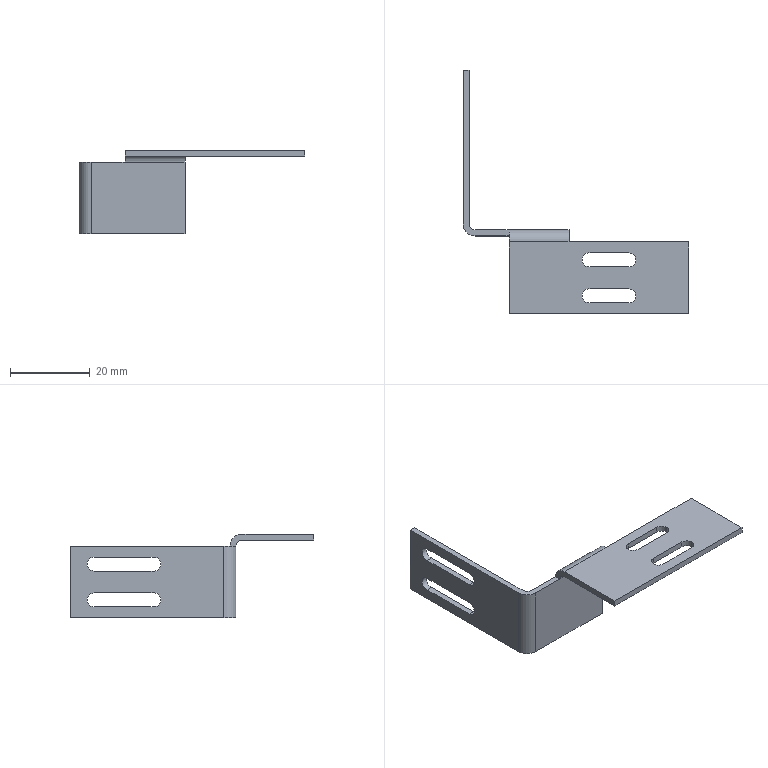Part | SolidWorks | features ICE 4, Fillet 2, ExtruThin 1 | 1 solid | 36 faces | box 56.5 x 61 x 21 mm | volume 2744 mm3 | plane 22 | cylinder 14 | commonest cylinder face diameters 3.5 x10 3 x2 6 x2
STEP:
#1=CARTESIAN_POINT('',(40.,-14.75,19.5));
#2=VERTEX_POINT('',#1);
#3=CARTESIAN_POINT('',(41.75,-16.5,19.5));
#4=VERTEX_POINT('',#3);
#5=CARTESIAN_POINT('',(40.,-16.5,19.5));
#6=DIRECTION('',(0.,0.,-1.));
#7=DIRECTION('',(0.,1.,0.));
#8=AXIS2_PLACEMENT_3D('',#5,#6,#7);
#9=CIRCLE('',#8,1.75);
#10=EDGE_CURVE('',#2,#4,#9,.T.);
#11=ORIENTED_EDGE('',*,*,#10,.T.);
#12=CARTESIAN_POINT('',(41.75,-16.5,21.));
#13=VERTEX_POINT('',#12);
#14=CARTESIAN_POINT('',(41.75,-16.5,11.));
#15=DIRECTION('',(0.,0.,1.));
#16=VECTOR('',#15,1000.);
#17=LINE('',#14,#16);
#18=EDGE_CURVE('',#4,#13,#17,.T.);
#19=ORIENTED_EDGE('',*,*,#18,.T.);
#20=CARTESIAN_POINT('',(40.,-14.75,21.));
#21=VERTEX_POINT('',#20);
#22=CARTESIAN_POINT('',(40.,-16.5,21.));
#23=DIRECTION('',(0.,0.,1.));
#24=DIRECTION('',(-1.,0.,0.));
#25=AXIS2_PLACEMENT_3D('',#22,#23,#24);
#26=CIRCLE('',#25,1.75);
#27=EDGE_CURVE('',#13,#21,#26,.T.);
#28=ORIENTED_EDGE('',*,*,#27,.T.);
#29=CARTESIAN_POINT('',(40.,-14.75,11.));
#30=DIRECTION('',(0.,0.,1.));
#31=VECTOR('',#30,1000.);
#32=LINE('',#29,#31);
#33=EDGE_CURVE('',#2,#21,#32,.T.);
#34=ORIENTED_EDGE('',*,*,#33,.F.);
#35=EDGE_LOOP('',(#11,#19,#28,#34));
#36=FACE_OUTER_BOUND('',#35,.T.);
#37=CARTESIAN_POINT('',(40.,-16.5,11.));
#38=DIRECTION('',(0.,0.,1.));
#39=DIRECTION('',(1.,0.,0.));
#40=AXIS2_PLACEMENT_3D('',#37,#38,#39);
#41=CYLINDRICAL_SURFACE('',#40,1.75);
#42=ADVANCED_FACE('',(#36),#41,.F.);
#43=CARTESIAN_POINT('',(40.,-5.75,19.5));
#44=VERTEX_POINT('',#43);
#45=CARTESIAN_POINT('',(41.75,-7.5,19.5));
#46=VERTEX_POINT('',#45);
#47=CARTESIAN_POINT('',(40.,-7.5,19.5));
#48=DIRECTION('',(0.,0.,-1.));
#49=DIRECTION('',(0.,1.,0.));
#50=AXIS2_PLACEMENT_3D('',#47,#48,#49);
#51=CIRCLE('',#50,1.75);
#52=EDGE_CURVE('',#44,#46,#51,.T.);
#53=ORIENTED_EDGE('',*,*,#52,.T.);
#54=CARTESIAN_POINT('',(41.75,-7.5,21.));
#55=VERTEX_POINT('',#54);
#56=CARTESIAN_POINT('',(41.75,-7.5,11.));
#57=DIRECTION('',(0.,0.,1.));
#58=VECTOR('',#57,1000.);
#59=LINE('',#56,#58);
#60=EDGE_CURVE('',#46,#55,#59,.T.);
#61=ORIENTED_EDGE('',*,*,#60,.T.);
#62=CARTESIAN_POINT('',(40.,-5.75,21.));
#63=VERTEX_POINT('',#62);
#64=CARTESIAN_POINT('',(40.,-7.5,21.));
#65=DIRECTION('',(0.,0.,1.));
#66=DIRECTION('',(1.,0.,0.));
#67=AXIS2_PLACEMENT_3D('',#64,#65,#66);
#68=CIRCLE('',#67,1.75);
#69=EDGE_CURVE('',#55,#63,#68,.T.);
#70=ORIENTED_EDGE('',*,*,#69,.T.);
#71=CARTESIAN_POINT('',(40.,-5.75,11.));
#72=DIRECTION('',(0.,0.,1.));
#73=VECTOR('',#72,1000.);
#74=LINE('',#71,#73);
#75=EDGE_CURVE('',#44,#63,#74,.T.);
#76=ORIENTED_EDGE('',*,*,#75,.F.);
#77=EDGE_LOOP('',(#53,#61,#70,#76));
#78=FACE_OUTER_BOUND('',#77,.T.);
#79=CARTESIAN_POINT('',(40.,-7.5,11.));
#80=DIRECTION('',(0.,0.,1.));
#81=DIRECTION('',(1.,0.,0.));
#82=AXIS2_PLACEMENT_3D('',#79,#80,#81);
#83=CYLINDRICAL_SURFACE('',#82,1.75);
#84=ADVANCED_FACE('',(#78),#83,.F.);
#85=CARTESIAN_POINT('',(10.,-3.,21.));
#86=VERTEX_POINT('',#85);
#87=CARTESIAN_POINT('',(25.,-3.,21.));
#88=VERTEX_POINT('',#87);
#89=CARTESIAN_POINT('',(10.,-3.,21.));
#90=DIRECTION('',(1.,0.,0.));
#91=VECTOR('',#90,1000.);
#92=LINE('',#89,#91);
#93=EDGE_CURVE('',#86,#88,#92,.T.);
#94=ORIENTED_EDGE('',*,*,#93,.T.);
#95=CARTESIAN_POINT('',(25.,0.,18.));
#96=VERTEX_POINT('',#95);
#97=CARTESIAN_POINT('',(25.,-3.,18.));
#98=DIRECTION('',(-1.,0.,0.));
#99=DIRECTION('',(0.,0.,-1.));
#100=AXIS2_PLACEMENT_3D('',#97,#98,#99);
#101=CIRCLE('',#100,3.);
#102=EDGE_CURVE('',#88,#96,#101,.T.);
#103=ORIENTED_EDGE('',*,*,#102,.T.);
#104=CARTESIAN_POINT('',(10.,0.,18.));
#105=VERTEX_POINT('',#104);
#106=CARTESIAN_POINT('',(10.,0.,18.));
#107=DIRECTION('',(1.,0.,0.));
#108=VECTOR('',#107,1000.);
#109=LINE('',#106,#108);
#110=EDGE_CURVE('',#105,#96,#109,.T.);
#111=ORIENTED_EDGE('',*,*,#110,.F.);
#112=CARTESIAN_POINT('',(10.,-3.,18.));
#113=DIRECTION('',(1.,0.,0.));
#114=DIRECTION('',(0.,0.,-1.));
#115=AXIS2_PLACEMENT_3D('',#112,#113,#114);
#116=CIRCLE('',#115,3.);
#117=EDGE_CURVE('',#105,#86,#116,.T.);
#118=ORIENTED_EDGE('',*,*,#117,.T.);
#119=EDGE_LOOP('',(#94,#103,#111,#118));
#120=FACE_OUTER_BOUND('',#119,.T.);
#121=CARTESIAN_POINT('',(10.,-3.,18.));
#122=DIRECTION('',(1.,0.,0.));
#123=DIRECTION('',(0.,0.,-1.));
#124=AXIS2_PLACEMENT_3D('',#121,#122,#123);
#125=CYLINDRICAL_SURFACE('',#124,3.);
#126=ADVANCED_FACE('',(#120),#125,.T.);
#127=CARTESIAN_POINT('',(10.,-1.5,18.));
#128=VERTEX_POINT('',#127);
#129=CARTESIAN_POINT('',(25.,-1.5,18.));
#130=VERTEX_POINT('',#129);
#131=CARTESIAN_POINT('',(10.,-1.5,18.));
#132=DIRECTION('',(1.,0.,0.));
#133=VECTOR('',#132,1000.);
#134=LINE('',#131,#133);
#135=EDGE_CURVE('',#128,#130,#134,.T.);
#136=ORIENTED_EDGE('',*,*,#135,.T.);
#137=CARTESIAN_POINT('',(25.,-3.,19.5));
#138=VERTEX_POINT('',#137);
#139=CARTESIAN_POINT('',(25.,-3.,18.));
#140=DIRECTION('',(1.,0.,0.));
#141=DIRECTION('',(0.,0.,-1.));
#142=AXIS2_PLACEMENT_3D('',#139,#140,#141);
#143=CIRCLE('',#142,1.5);
#144=EDGE_CURVE('',#130,#138,#143,.T.);
#145=ORIENTED_EDGE('',*,*,#144,.T.);
#146=CARTESIAN_POINT('',(10.,-3.,19.5));
#147=VERTEX_POINT('',#146);
#148=CARTESIAN_POINT('',(10.,-3.,19.5));
#149=DIRECTION('',(1.,0.,0.));
#150=VECTOR('',#149,1000.);
#151=LINE('',#148,#150);
#152=EDGE_CURVE('',#147,#138,#151,.T.);
#153=ORIENTED_EDGE('',*,*,#152,.F.);
#154=CARTESIAN_POINT('',(10.,-3.,18.));
#155=DIRECTION('',(-1.,0.,0.));
#156=DIRECTION('',(0.,0.,-1.));
#157=AXIS2_PLACEMENT_3D('',#154,#155,#156);
#158=CIRCLE('',#157,1.5);
#159=EDGE_CURVE('',#147,#128,#158,.T.);
#160=ORIENTED_EDGE('',*,*,#159,.T.);
#161=EDGE_LOOP('',(#136,#145,#153,#160));
#162=FACE_OUTER_BOUND('',#161,.T.);
#163=CARTESIAN_POINT('',(10.,-3.,18.));
#164=DIRECTION('',(1.,0.,0.));
#165=DIRECTION('',(0.,0.,-1.));
#166=AXIS2_PLACEMENT_3D('',#163,#164,#165);
#167=CYLINDRICAL_SURFACE('',#166,1.5);
#168=ADVANCED_FACE('',(#162),#167,.F.);
#169=CARTESIAN_POINT('',(1.5,-1.5,18.));
#170=VERTEX_POINT('',#169);
#171=CARTESIAN_POINT('',(0.,-1.5,18.));
#172=DIRECTION('',(1.,0.,0.));
#173=VECTOR('',#172,1000.);
#174=LINE('',#171,#173);
#175=EDGE_CURVE('',#170,#128,#174,.T.);
#176=ORIENTED_EDGE('',*,*,#175,.F.);
#177=CARTESIAN_POINT('',(1.5,-1.5,0.));
#178=VERTEX_POINT('',#177);
#179=CARTESIAN_POINT('',(1.5,-1.5,18.));
#180=DIRECTION('',(0.,0.,-1.));
#181=VECTOR('',#180,1000.);
#182=LINE('',#179,#181);
#183=EDGE_CURVE('',#170,#178,#182,.T.);
#184=ORIENTED_EDGE('',*,*,#183,.T.);
#185=CARTESIAN_POINT('',(25.,-1.5,0.));
#186=VERTEX_POINT('',#185);
#187=CARTESIAN_POINT('',(0.,-1.5,0.));
#188=DIRECTION('',(1.,0.,0.));
#189=VECTOR('',#188,1000.);
#190=LINE('',#187,#189);
#191=EDGE_CURVE('',#178,#186,#190,.T.);
#192=ORIENTED_EDGE('',*,*,#191,.T.);
#193=CARTESIAN_POINT('',(25.,-1.5,18.));
#194=DIRECTION('',(0.,0.,-1.));
#195=VECTOR('',#194,1000.);
#196=LINE('',#193,#195);
#197=EDGE_CURVE('',#130,#186,#196,.T.);
#198=ORIENTED_EDGE('',*,*,#197,.F.);
#199=ORIENTED_EDGE('',*,*,#135,.F.);
#200=EDGE_LOOP('',(#176,#184,#192,#198,#199));
#201=FACE_OUTER_BOUND('',#200,.T.);
#202=CARTESIAN_POINT('',(0.,-1.5,18.));
#203=DIRECTION('',(0.,1.,0.));
#204=DIRECTION('',(0.,0.,1.));
#205=AXIS2_PLACEMENT_3D('',#202,#203,#204);
#206=PLANE('',#205);
#207=ADVANCED_FACE('',(#201),#206,.F.);
#208=CARTESIAN_POINT('',(25.,0.,0.));
#209=VERTEX_POINT('',#208);
#210=CARTESIAN_POINT('',(25.,0.,0.));
#211=DIRECTION('',(0.,-1.,0.));
#212=VECTOR('',#211,1000.);
#213=LINE('',#210,#212);
#214=EDGE_CURVE('',#209,#186,#213,.T.);
#215=ORIENTED_EDGE('',*,*,#214,.F.);
#216=CARTESIAN_POINT('',(25.,0.,18.));
#217=DIRECTION('',(0.,0.,-1.));
#218=VECTOR('',#217,1000.);
#219=LINE('',#216,#218);
#220=EDGE_CURVE('',#96,#209,#219,.T.);
#221=ORIENTED_EDGE('',*,*,#220,.F.);
#222=ORIENTED_EDGE('',*,*,#102,.F.);
#223=CARTESIAN_POINT('',(25.,-3.,21.));
#224=DIRECTION('',(0.,0.,1.));
#225=VECTOR('',#224,1000.);
#226=LINE('',#223,#225);
#227=EDGE_CURVE('',#138,#88,#226,.T.);
#228=ORIENTED_EDGE('',*,*,#227,.F.);
#229=ORIENTED_EDGE('',*,*,#144,.F.);
#230=ORIENTED_EDGE('',*,*,#197,.T.);
#231=EDGE_LOOP('',(#215,#221,#222,#228,#229,#230));
#232=FACE_OUTER_BOUND('',#231,.T.);
#233=CARTESIAN_POINT('',(25.,0.,18.));
#234=DIRECTION('',(1.,0.,0.));
#235=DIRECTION('',(0.,0.,-1.));
#236=AXIS2_PLACEMENT_3D('',#233,#234,#235);
#237=PLANE('',#236);
#238=ADVANCED_FACE('',(#232),#237,.T.);
#239=CARTESIAN_POINT('',(1.5,0.,0.));
#240=VERTEX_POINT('',#239);
#241=CARTESIAN_POINT('',(0.,0.,0.));
#242=DIRECTION('',(1.,0.,0.));
#243=VECTOR('',#242,1000.);
#244=LINE('',#241,#243);
#245=EDGE_CURVE('',#240,#209,#244,.T.);
#246=ORIENTED_EDGE('',*,*,#245,.F.);
#247=CARTESIAN_POINT('',(1.5,0.,18.));
#248=VERTEX_POINT('',#247);
#249=CARTESIAN_POINT('',(1.5,0.,18.));
#250=DIRECTION('',(0.,0.,1.));
#251=VECTOR('',#250,1000.);
#252=LINE('',#249,#251);
#253=EDGE_CURVE('',#240,#248,#252,.T.);
#254=ORIENTED_EDGE('',*,*,#253,.T.);
#255=CARTESIAN_POINT('',(0.,0.,18.));
#256=DIRECTION('',(1.,0.,0.));
#257=VECTOR('',#256,1000.);
#258=LINE('',#255,#257);
#259=EDGE_CURVE('',#248,#105,#258,.T.);
#260=ORIENTED_EDGE('',*,*,#259,.T.);
#261=ORIENTED_EDGE('',*,*,#110,.T.);
#262=ORIENTED_EDGE('',*,*,#220,.T.);
#263=EDGE_LOOP('',(#246,#254,#260,#261,#262));
#264=FACE_OUTER_BOUND('',#263,.T.);
#265=CARTESIAN_POINT('',(0.,0.,18.));
#266=DIRECTION('',(0.,1.,0.));
#267=DIRECTION('',(0.,0.,1.));
#268=AXIS2_PLACEMENT_3D('',#265,#266,#267);
#269=PLANE('',#268);
#270=ADVANCED_FACE('',(#264),#269,.T.);
#271=CARTESIAN_POINT('',(0.,34.,11.75));
#272=VERTEX_POINT('',#271);
#273=CARTESIAN_POINT('',(0.,34.,15.25));
#274=VERTEX_POINT('',#273);
#275=CARTESIAN_POINT('',(0.,34.,13.5));
#276=DIRECTION('',(1.,0.,0.));
#277=DIRECTION('',(0.,0.,-1.));
#278=AXIS2_PLACEMENT_3D('',#275,#276,#277);
#279=CIRCLE('',#278,1.75);
#280=EDGE_CURVE('',#272,#274,#279,.T.);
#281=ORIENTED_EDGE('',*,*,#280,.F.);
#282=CARTESIAN_POINT('',(0.,19.,11.75));
#283=VERTEX_POINT('',#282);
#284=CARTESIAN_POINT('',(0.,0.,11.75));
#285=DIRECTION('',(0.,1.,0.));
#286=VECTOR('',#285,1000.);
#287=LINE('',#284,#286);
#288=EDGE_CURVE('',#283,#272,#287,.T.);
#289=ORIENTED_EDGE('',*,*,#288,.F.);
#290=CARTESIAN_POINT('',(0.,19.,15.25));
#291=VERTEX_POINT('',#290);
#292=CARTESIAN_POINT('',(0.,19.,13.5));
#293=DIRECTION('',(1.,0.,0.));
#294=DIRECTION('',(0.,0.,-1.));
#295=AXIS2_PLACEMENT_3D('',#292,#293,#294);
#296=CIRCLE('',#295,1.75);
#297=EDGE_CURVE('',#291,#283,#296,.T.);
#298=ORIENTED_EDGE('',*,*,#297,.F.);
#299=CARTESIAN_POINT('',(0.,0.,15.25));
#300=DIRECTION('',(0.,-1.,0.));
#301=VECTOR('',#300,1000.);
#302=LINE('',#299,#301);
#303=EDGE_CURVE('',#274,#291,#302,.T.);
#304=ORIENTED_EDGE('',*,*,#303,.F.);
#305=EDGE_LOOP('',(#281,#289,#298,#304));
#306=FACE_BOUND('',#305,.T.);
#307=CARTESIAN_POINT('',(0.,34.,2.75));
#308=VERTEX_POINT('',#307);
#309=CARTESIAN_POINT('',(0.,34.,6.25));
#310=VERTEX_POINT('',#309);
#311=CARTESIAN_POINT('',(0.,34.,4.5));
#312=DIRECTION('',(1.,0.,0.));
#313=DIRECTION('',(0.,0.,-1.));
#314=AXIS2_PLACEMENT_3D('',#311,#312,#313);
#315=CIRCLE('',#314,1.75);
#316=EDGE_CURVE('',#308,#310,#315,.T.);
#317=ORIENTED_EDGE('',*,*,#316,.F.);
#318=CARTESIAN_POINT('',(0.,19.,2.75));
#319=VERTEX_POINT('',#318);
#320=CARTESIAN_POINT('',(0.,0.,2.75));
#321=DIRECTION('',(0.,1.,0.));
#322=VECTOR('',#321,1000.);
#323=LINE('',#320,#322);
#324=EDGE_CURVE('',#319,#308,#323,.T.);
#325=ORIENTED_EDGE('',*,*,#324,.F.);
#326=CARTESIAN_POINT('',(0.,19.,6.25));
#327=VERTEX_POINT('',#326);
#328=CARTESIAN_POINT('',(0.,19.,4.5));
#329=DIRECTION('',(1.,0.,0.));
#330=DIRECTION('',(0.,0.,-1.));
#331=AXIS2_PLACEMENT_3D('',#328,#329,#330);
#332=CIRCLE('',#331,1.75);
#333=EDGE_CURVE('',#327,#319,#332,.T.);
#334=ORIENTED_EDGE('',*,*,#333,.F.);
#335=CARTESIAN_POINT('',(0.,0.,6.25));
#336=DIRECTION('',(0.,-1.,0.));
#337=VECTOR('',#336,1000.);
#338=LINE('',#335,#337);
#339=EDGE_CURVE('',#310,#327,#338,.T.);
#340=ORIENTED_EDGE('',*,*,#339,.F.);
#341=EDGE_LOOP('',(#317,#325,#334,#340));
#342=FACE_BOUND('',#341,.T.);
#343=CARTESIAN_POINT('',(0.,40.,18.));
#344=VERTEX_POINT('',#343);
#345=CARTESIAN_POINT('',(0.,1.5,18.));
#346=VERTEX_POINT('',#345);
#347=CARTESIAN_POINT('',(0.,0.,18.));
#348=DIRECTION('',(0.,-1.,0.));
#349=VECTOR('',#348,1000.);
#350=LINE('',#347,#349);
#351=EDGE_CURVE('',#344,#346,#350,.T.);
#352=ORIENTED_EDGE('',*,*,#351,.T.);
#353=CARTESIAN_POINT('',(0.,1.5,0.));
#354=VERTEX_POINT('',#353);
#355=CARTESIAN_POINT('',(0.,1.5,0.));
#356=DIRECTION('',(0.,0.,-1.));
#357=VECTOR('',#356,1000.);
#358=LINE('',#355,#357);
#359=EDGE_CURVE('',#346,#354,#358,.T.);
#360=ORIENTED_EDGE('',*,*,#359,.T.);
#361=CARTESIAN_POINT('',(0.,40.,0.));
#362=VERTEX_POINT('',#361);
#363=CARTESIAN_POINT('',(0.,0.,0.));
#364=DIRECTION('',(0.,-1.,0.));
#365=VECTOR('',#364,1000.);
#366=LINE('',#363,#365);
#367=EDGE_CURVE('',#362,#354,#366,.T.);
#368=ORIENTED_EDGE('',*,*,#367,.F.);
#369=CARTESIAN_POINT('',(0.,40.,18.));
#370=DIRECTION('',(0.,0.,-1.));
#371=VECTOR('',#370,1000.);
#372=LINE('',#369,#371);
#373=EDGE_CURVE('',#344,#362,#372,.T.);
#374=ORIENTED_EDGE('',*,*,#373,.F.);
#375=EDGE_LOOP('',(#352,#360,#368,#374));
#376=FACE_OUTER_BOUND('',#375,.T.);
#377=CARTESIAN_POINT('',(0.,0.,18.));
#378=DIRECTION('',(1.,0.,0.));
#379=DIRECTION('',(0.,0.,-1.));
#380=AXIS2_PLACEMENT_3D('',#377,#378,#379);
#381=PLANE('',#380);
#382=ADVANCED_FACE('',(#306,#342,#376),#381,.T.);
#383=CARTESIAN_POINT('',(-1.5,40.,0.));
#384=VERTEX_POINT('',#383);
#385=CARTESIAN_POINT('',(-1.5,40.,0.));
#386=DIRECTION('',(1.,0.,0.));
#387=VECTOR('',#386,1000.);
#388=LINE('',#385,#387);
#389=EDGE_CURVE('',#384,#362,#388,.T.);
#390=ORIENTED_EDGE('',*,*,#389,.F.);
#391=CARTESIAN_POINT('',(-1.5,40.,18.));
#392=VERTEX_POINT('',#391);
#393=CARTESIAN_POINT('',(-1.5,40.,18.));
#394=DIRECTION('',(0.,0.,-1.));
#395=VECTOR('',#394,1000.);
#396=LINE('',#393,#395);
#397=EDGE_CURVE('',#392,#384,#396,.T.);
#398=ORIENTED_EDGE('',*,*,#397,.F.);
#399=CARTESIAN_POINT('',(-1.5,40.,18.));
#400=DIRECTION('',(1.,0.,0.));
#401=VECTOR('',#400,1000.);
#402=LINE('',#399,#401);
#403=EDGE_CURVE('',#392,#344,#402,.T.);
#404=ORIENTED_EDGE('',*,*,#403,.T.);
#405=ORIENTED_EDGE('',*,*,#373,.T.);
#406=EDGE_LOOP('',(#390,#398,#404,#405));
#407=FACE_OUTER_BOUND('',#406,.T.);
#408=CARTESIAN_POINT('',(-1.5,40.,18.));
#409=DIRECTION('',(0.,1.,0.));
#410=DIRECTION('',(0.,0.,1.));
#411=AXIS2_PLACEMENT_3D('',#408,#409,#410);
#412=PLANE('',#411);
#413=ADVANCED_FACE('',(#407),#412,.T.);
#414=CARTESIAN_POINT('',(-1.5,34.,11.75));
#415=VERTEX_POINT('',#414);
#416=CARTESIAN_POINT('',(-1.5,19.,11.75));
#417=VERTEX_POINT('',#416);
#418=CARTESIAN_POINT('',(-1.5,34.,11.75));
#419=DIRECTION('',(0.,-1.,0.));
#420=VECTOR('',#419,1000.);
#421=LINE('',#418,#420);
#422=EDGE_CURVE('',#415,#417,#421,.T.);
#423=ORIENTED_EDGE('',*,*,#422,.F.);
#424=CARTESIAN_POINT('',(-1.5,34.,15.25));
#425=VERTEX_POINT('',#424);
#426=CARTESIAN_POINT('',(-1.5,34.,13.5));
#427=DIRECTION('',(-1.,0.,0.));
#428=DIRECTION('',(0.,0.,-1.));
#429=AXIS2_PLACEMENT_3D('',#426,#427,#428);
#430=CIRCLE('',#429,1.75);
#431=EDGE_CURVE('',#425,#415,#430,.T.);
#432=ORIENTED_EDGE('',*,*,#431,.F.);
#433=CARTESIAN_POINT('',(-1.5,19.,15.25));
#434=VERTEX_POINT('',#433);
#435=CARTESIAN_POINT('',(-1.5,34.,15.25));
#436=DIRECTION('',(0.,1.,0.));
#437=VECTOR('',#436,1000.);
#438=LINE('',#435,#437);
#439=EDGE_CURVE('',#434,#425,#438,.T.);
#440=ORIENTED_EDGE('',*,*,#439,.F.);
#441=CARTESIAN_POINT('',(-1.5,19.,13.5));
#442=DIRECTION('',(-1.,0.,0.));
#443=DIRECTION('',(0.,0.,-1.));
#444=AXIS2_PLACEMENT_3D('',#441,#442,#443);
#445=CIRCLE('',#444,1.75);
#446=EDGE_CURVE('',#417,#434,#445,.T.);
#447=ORIENTED_EDGE('',*,*,#446,.F.);
#448=EDGE_LOOP('',(#423,#432,#440,#447));
#449=FACE_BOUND('',#448,.T.);
#450=CARTESIAN_POINT('',(-1.5,34.,2.75));
#451=VERTEX_POINT('',#450);
#452=CARTESIAN_POINT('',(-1.5,19.,2.75));
#453=VERTEX_POINT('',#452);
#454=CARTESIAN_POINT('',(-1.5,34.,2.75));
#455=DIRECTION('',(0.,-1.,0.));
#456=VECTOR('',#455,1000.);
#457=LINE('',#454,#456);
#458=EDGE_CURVE('',#451,#453,#457,.T.);
#459=ORIENTED_EDGE('',*,*,#458,.F.);
#460=CARTESIAN_POINT('',(-1.5,34.,6.25));
#461=VERTEX_POINT('',#460);
#462=CARTESIAN_POINT('',(-1.5,34.,4.5));
#463=DIRECTION('',(-1.,0.,0.));
#464=DIRECTION('',(0.,0.,1.));
#465=AXIS2_PLACEMENT_3D('',#462,#463,#464);
#466=CIRCLE('',#465,1.75);
#467=EDGE_CURVE('',#461,#451,#466,.T.);
#468=ORIENTED_EDGE('',*,*,#467,.F.);
#469=CARTESIAN_POINT('',(-1.5,19.,6.25));
#470=VERTEX_POINT('',#469);
#471=CARTESIAN_POINT('',(-1.5,34.,6.25));
#472=DIRECTION('',(0.,1.,0.));
#473=VECTOR('',#472,1000.);
#474=LINE('',#471,#473);
#475=EDGE_CURVE('',#470,#461,#474,.T.);
#476=ORIENTED_EDGE('',*,*,#475,.F.);
#477=CARTESIAN_POINT('',(-1.5,19.,4.5));
#478=DIRECTION('',(-1.,0.,0.));
#479=DIRECTION('',(0.,0.,1.));
#480=AXIS2_PLACEMENT_3D('',#477,#478,#479);
#481=CIRCLE('',#480,1.75);
#482=EDGE_CURVE('',#453,#470,#481,.T.);
#483=ORIENTED_EDGE('',*,*,#482,.F.);
#484=EDGE_LOOP('',(#459,#468,#476,#483));
#485=FACE_BOUND('',#484,.T.);
#486=CARTESIAN_POINT('',(-1.5,1.5,0.));
#487=VERTEX_POINT('',#486);
#488=CARTESIAN_POINT('',(-1.5,0.,0.));
#489=DIRECTION('',(0.,-1.,0.));
#490=VECTOR('',#489,1000.);
#491=LINE('',#488,#490);
#492=EDGE_CURVE('',#384,#487,#491,.T.);
#493=ORIENTED_EDGE('',*,*,#492,.T.);
#494=CARTESIAN_POINT('',(-1.5,1.5,18.));
#495=VERTEX_POINT('',#494);
#496=CARTESIAN_POINT('',(-1.5,1.5,18.));
#497=DIRECTION('',(0.,0.,1.));
#498=VECTOR('',#497,1000.);
#499=LINE('',#496,#498);
#500=EDGE_CURVE('',#487,#495,#499,.T.);
#501=ORIENTED_EDGE('',*,*,#500,.T.);
#502=CARTESIAN_POINT('',(-1.5,0.,18.));
#503=DIRECTION('',(0.,-1.,0.));
#504=VECTOR('',#503,1000.);
#505=LINE('',#502,#504);
#506=EDGE_CURVE('',#392,#495,#505,.T.);
#507=ORIENTED_EDGE('',*,*,#506,.F.);
#508=ORIENTED_EDGE('',*,*,#397,.T.);
#509=EDGE_LOOP('',(#493,#501,#507,#508));
#510=FACE_OUTER_BOUND('',#509,.T.);
#511=CARTESIAN_POINT('',(-1.5,0.,18.));
#512=DIRECTION('',(1.,0.,0.));
#513=DIRECTION('',(0.,0.,-1.));
#514=AXIS2_PLACEMENT_3D('',#511,#512,#513);
#515=PLANE('',#514);
#516=ADVANCED_FACE('',(#449,#485,#510),#515,.F.);
#517=ORIENTED_EDGE('',*,*,#175,.T.);
#518=CARTESIAN_POINT('',(10.,0.,18.));
#519=DIRECTION('',(0.,1.,0.));
#520=VECTOR('',#519,1000.);
#521=LINE('',#518,#520);
#522=EDGE_CURVE('',#128,#105,#521,.T.);
#523=ORIENTED_EDGE('',*,*,#522,.T.);
#524=ORIENTED_EDGE('',*,*,#259,.F.);
#525=CARTESIAN_POINT('',(1.5,1.5,18.));
#526=DIRECTION('',(0.,0.,-1.));
#527=DIRECTION('',(-1.,0.,0.));
#528=AXIS2_PLACEMENT_3D('',#525,#526,#527);
#529=CIRCLE('',#528,1.5);
#530=EDGE_CURVE('',#248,#346,#529,.T.);
#531=ORIENTED_EDGE('',*,*,#530,.T.);
#532=ORIENTED_EDGE('',*,*,#351,.F.);
#533=ORIENTED_EDGE('',*,*,#403,.F.);
#534=ORIENTED_EDGE('',*,*,#506,.T.);
#535=CARTESIAN_POINT('',(1.5,1.5,18.));
#536=DIRECTION('',(0.,0.,1.));
#537=DIRECTION('',(-1.,0.,0.));
#538=AXIS2_PLACEMENT_3D('',#535,#536,#537);
#539=CIRCLE('',#538,3.);
#540=EDGE_CURVE('',#495,#170,#539,.T.);
#541=ORIENTED_EDGE('',*,*,#540,.T.);
#542=EDGE_LOOP('',(#517,#523,#524,#531,#532,#533,#534,#541));
#543=FACE_OUTER_BOUND('',#542,.T.);
#544=CARTESIAN_POINT('',(25.,-1.5,18.));
#545=DIRECTION('',(0.,0.,-1.));
#546=DIRECTION('',(-1.,0.,0.));
#547=AXIS2_PLACEMENT_3D('',#544,#545,#546);
#548=PLANE('',#547);
#549=ADVANCED_FACE('',(#543),#548,.F.);
#550=ORIENTED_EDGE('',*,*,#191,.F.);
#551=CARTESIAN_POINT('',(1.5,1.5,0.));
#552=DIRECTION('',(0.,0.,-1.));
#553=DIRECTION('',(-1.,0.,0.));
#554=AXIS2_PLACEMENT_3D('',#551,#552,#553);
#555=CIRCLE('',#554,3.);
#556=EDGE_CURVE('',#178,#487,#555,.T.);
#557=ORIENTED_EDGE('',*,*,#556,.T.);
#558=ORIENTED_EDGE('',*,*,#492,.F.);
#559=ORIENTED_EDGE('',*,*,#389,.T.);
#560=ORIENTED_EDGE('',*,*,#367,.T.);
#561=CARTESIAN_POINT('',(1.5,1.5,0.));
#562=DIRECTION('',(0.,0.,1.));
#563=DIRECTION('',(-1.,0.,0.));
#564=AXIS2_PLACEMENT_3D('',#561,#562,#563);
#565=CIRCLE('',#564,1.5);
#566=EDGE_CURVE('',#354,#240,#565,.T.);
#567=ORIENTED_EDGE('',*,*,#566,.T.);
#568=ORIENTED_EDGE('',*,*,#245,.T.);
#569=ORIENTED_EDGE('',*,*,#214,.T.);
#570=EDGE_LOOP('',(#550,#557,#558,#559,#560,#567,#568,#569));
#571=FACE_OUTER_BOUND('',#570,.T.);
#572=CARTESIAN_POINT('',(25.,-1.5,0.));
#573=DIRECTION('',(0.,0.,-1.));
#574=DIRECTION('',(-1.,0.,0.));
#575=AXIS2_PLACEMENT_3D('',#572,#573,#574);
#576=PLANE('',#575);
#577=ADVANCED_FACE('',(#571),#576,.T.);
#578=ORIENTED_EDGE('',*,*,#530,.F.);
#579=ORIENTED_EDGE('',*,*,#253,.F.);
#580=ORIENTED_EDGE('',*,*,#566,.F.);
#581=ORIENTED_EDGE('',*,*,#359,.F.);
#582=EDGE_LOOP('',(#578,#579,#580,#581));
#583=FACE_OUTER_BOUND('',#582,.T.);
#584=CARTESIAN_POINT('',(1.5,1.5,18.));
#585=DIRECTION('',(0.,0.,1.));
#586=DIRECTION('',(1.,0.,0.));
#587=AXIS2_PLACEMENT_3D('',#584,#585,#586);
#588=CYLINDRICAL_SURFACE('',#587,1.5);
#589=ADVANCED_FACE('',(#583),#588,.F.);
#590=ORIENTED_EDGE('',*,*,#540,.F.);
#591=ORIENTED_EDGE('',*,*,#500,.F.);
#592=ORIENTED_EDGE('',*,*,#556,.F.);
#593=ORIENTED_EDGE('',*,*,#183,.F.);
#594=EDGE_LOOP('',(#590,#591,#592,#593));
#595=FACE_OUTER_BOUND('',#594,.T.);
#596=CARTESIAN_POINT('',(1.5,1.5,18.));
#597=DIRECTION('',(0.,0.,-1.));
#598=DIRECTION('',(-1.,0.,0.));
#599=AXIS2_PLACEMENT_3D('',#596,#597,#598);
#600=CYLINDRICAL_SURFACE('',#599,3.);
#601=ADVANCED_FACE('',(#595),#600,.T.);
#602=CARTESIAN_POINT('',(30.,-18.25,19.5));
#603=VERTEX_POINT('',#602);
#604=CARTESIAN_POINT('',(30.,-14.75,19.5));
#605=VERTEX_POINT('',#604);
#606=CARTESIAN_POINT('',(30.,-16.5,19.5));
#607=DIRECTION('',(0.,0.,-1.));
#608=DIRECTION('',(0.,1.,0.));
#609=AXIS2_PLACEMENT_3D('',#606,#607,#608);
#610=CIRCLE('',#609,1.75);
#611=EDGE_CURVE('',#603,#605,#610,.T.);
#612=ORIENTED_EDGE('',*,*,#611,.F.);
#613=CARTESIAN_POINT('',(40.,-18.25,19.5));
#614=VERTEX_POINT('',#613);
#615=CARTESIAN_POINT('',(10.,-18.25,19.5));
#616=DIRECTION('',(-1.,0.,0.));
#617=VECTOR('',#616,1000.);
#618=LINE('',#615,#617);
#619=EDGE_CURVE('',#614,#603,#618,.T.);
#620=ORIENTED_EDGE('',*,*,#619,.F.);
#621=CARTESIAN_POINT('',(40.,-16.5,19.5));
#622=DIRECTION('',(0.,0.,-1.));
#623=DIRECTION('',(0.,1.,0.));
#624=AXIS2_PLACEMENT_3D('',#621,#622,#623);
#625=CIRCLE('',#624,1.75);
#626=EDGE_CURVE('',#4,#614,#625,.T.);
#627=ORIENTED_EDGE('',*,*,#626,.F.);
#628=ORIENTED_EDGE('',*,*,#10,.F.);
#629=CARTESIAN_POINT('',(10.,-14.75,19.5));
#630=DIRECTION('',(1.,0.,0.));
#631=VECTOR('',#630,1000.);
#632=LINE('',#629,#631);
#633=EDGE_CURVE('',#605,#2,#632,.T.);
#634=ORIENTED_EDGE('',*,*,#633,.F.);
#635=EDGE_LOOP('',(#612,#620,#627,#628,#634));
#636=FACE_BOUND('',#635,.T.);
#637=CARTESIAN_POINT('',(30.,-9.25,19.5));
#638=VERTEX_POINT('',#637);
#639=CARTESIAN_POINT('',(30.,-5.75,19.5));
#640=VERTEX_POINT('',#639);
#641=CARTESIAN_POINT('',(30.,-7.5,19.5));
#642=DIRECTION('',(0.,0.,-1.));
#643=DIRECTION('',(0.,1.,0.));
#644=AXIS2_PLACEMENT_3D('',#641,#642,#643);
#645=CIRCLE('',#644,1.75);
#646=EDGE_CURVE('',#638,#640,#645,.T.);
#647=ORIENTED_EDGE('',*,*,#646,.F.);
#648=CARTESIAN_POINT('',(40.,-9.25,19.5));
#649=VERTEX_POINT('',#648);
#650=CARTESIAN_POINT('',(10.,-9.25,19.5));
#651=DIRECTION('',(-1.,0.,0.));
#652=VECTOR('',#651,1000.);
#653=LINE('',#650,#652);
#654=EDGE_CURVE('',#649,#638,#653,.T.);
#655=ORIENTED_EDGE('',*,*,#654,.F.);
#656=CARTESIAN_POINT('',(40.,-7.5,19.5));
#657=DIRECTION('',(0.,0.,-1.));
#658=DIRECTION('',(0.,1.,0.));
#659=AXIS2_PLACEMENT_3D('',#656,#657,#658);
#660=CIRCLE('',#659,1.75);
#661=EDGE_CURVE('',#46,#649,#660,.T.);
#662=ORIENTED_EDGE('',*,*,#661,.F.);
#663=ORIENTED_EDGE('',*,*,#52,.F.);
#664=CARTESIAN_POINT('',(10.,-5.75,19.5));
#665=DIRECTION('',(1.,0.,0.));
#666=VECTOR('',#665,1000.);
#667=LINE('',#664,#666);
#668=EDGE_CURVE('',#640,#44,#667,.T.);
#669=ORIENTED_EDGE('',*,*,#668,.F.);
#670=EDGE_LOOP('',(#647,#655,#662,#663,#669));
#671=FACE_BOUND('',#670,.T.);
#672=ORIENTED_EDGE('',*,*,#152,.T.);
#673=CARTESIAN_POINT('',(55.,-3.,19.5));
#674=VERTEX_POINT('',#673);
#675=CARTESIAN_POINT('',(10.,-3.,19.5));
#676=DIRECTION('',(-1.,0.,0.));
#677=VECTOR('',#676,1000.);
#678=LINE('',#675,#677);
#679=EDGE_CURVE('',#674,#138,#678,.T.);
#680=ORIENTED_EDGE('',*,*,#679,.F.);
#681=CARTESIAN_POINT('',(55.,-21.,19.5));
#682=VERTEX_POINT('',#681);
#683=CARTESIAN_POINT('',(55.,-3.,19.5));
#684=DIRECTION('',(0.,1.,0.));
#685=VECTOR('',#684,1000.);
#686=LINE('',#683,#685);
#687=EDGE_CURVE('',#682,#674,#686,.T.);
#688=ORIENTED_EDGE('',*,*,#687,.F.);
#689=CARTESIAN_POINT('',(10.,-21.,19.5));
#690=VERTEX_POINT('',#689);
#691=CARTESIAN_POINT('',(10.,-21.,19.5));
#692=DIRECTION('',(1.,0.,0.));
#693=VECTOR('',#692,1000.);
#694=LINE('',#691,#693);
#695=EDGE_CURVE('',#690,#682,#694,.T.);
#696=ORIENTED_EDGE('',*,*,#695,.F.);
#697=CARTESIAN_POINT('',(10.,-3.,19.5));
#698=DIRECTION('',(0.,1.,0.));
#699=VECTOR('',#698,1000.);
#700=LINE('',#697,#699);
#701=EDGE_CURVE('',#690,#147,#700,.T.);
#702=ORIENTED_EDGE('',*,*,#701,.T.);
#703=EDGE_LOOP('',(#672,#680,#688,#696,#702));
#704=FACE_OUTER_BOUND('',#703,.T.);
#705=CARTESIAN_POINT('',(10.,-3.,19.5));
#706=DIRECTION('',(0.,0.,-1.));
#707=DIRECTION('',(0.,1.,0.));
#708=AXIS2_PLACEMENT_3D('',#705,#706,#707);
#709=PLANE('',#708);
#710=ADVANCED_FACE('',(#636,#671,#704),#709,.T.);
#711=ORIENTED_EDGE('',*,*,#695,.T.);
#712=CARTESIAN_POINT('',(55.,-21.,21.));
#713=VERTEX_POINT('',#712);
#714=CARTESIAN_POINT('',(55.,-21.,21.));
#715=DIRECTION('',(0.,0.,-1.));
#716=VECTOR('',#715,1000.);
#717=LINE('',#714,#716);
#718=EDGE_CURVE('',#713,#682,#717,.T.);
#719=ORIENTED_EDGE('',*,*,#718,.F.);
#720=CARTESIAN_POINT('',(10.,-21.,21.));
#721=VERTEX_POINT('',#720);
#722=CARTESIAN_POINT('',(10.,-21.,21.));
#723=DIRECTION('',(1.,0.,0.));
#724=VECTOR('',#723,1000.);
#725=LINE('',#722,#724);
#726=EDGE_CURVE('',#721,#713,#725,.T.);
#727=ORIENTED_EDGE('',*,*,#726,.F.);
#728=CARTESIAN_POINT('',(10.,-21.,21.));
#729=DIRECTION('',(0.,0.,-1.));
#730=VECTOR('',#729,1000.);
#731=LINE('',#728,#730);
#732=EDGE_CURVE('',#721,#690,#731,.T.);
#733=ORIENTED_EDGE('',*,*,#732,.T.);
#734=EDGE_LOOP('',(#711,#719,#727,#733));
#735=FACE_OUTER_BOUND('',#734,.T.);
#736=CARTESIAN_POINT('',(10.,-21.,21.));
#737=DIRECTION('',(0.,-1.,0.));
#738=DIRECTION('',(0.,0.,-1.));
#739=AXIS2_PLACEMENT_3D('',#736,#737,#738);
#740=PLANE('',#739);
#741=ADVANCED_FACE('',(#735),#740,.T.);
#742=CARTESIAN_POINT('',(30.,-14.75,21.));
#743=VERTEX_POINT('',#742);
#744=CARTESIAN_POINT('',(30.,-18.25,21.));
#745=VERTEX_POINT('',#744);
#746=CARTESIAN_POINT('',(30.,-16.5,21.));
#747=DIRECTION('',(0.,0.,1.));
#748=DIRECTION('',(-1.,0.,0.));
#749=AXIS2_PLACEMENT_3D('',#746,#747,#748);
#750=CIRCLE('',#749,1.75);
#751=EDGE_CURVE('',#743,#745,#750,.T.);
#752=ORIENTED_EDGE('',*,*,#751,.F.);
#753=CARTESIAN_POINT('',(30.,-14.75,21.));
#754=DIRECTION('',(-1.,0.,0.));
#755=VECTOR('',#754,1000.);
#756=LINE('',#753,#755);
#757=EDGE_CURVE('',#21,#743,#756,.T.);
#758=ORIENTED_EDGE('',*,*,#757,.F.);
#759=ORIENTED_EDGE('',*,*,#27,.F.);
#760=CARTESIAN_POINT('',(40.,-18.25,21.));
#761=VERTEX_POINT('',#760);
#762=CARTESIAN_POINT('',(40.,-16.5,21.));
#763=DIRECTION('',(0.,0.,1.));
#764=DIRECTION('',(-1.,0.,0.));
#765=AXIS2_PLACEMENT_3D('',#762,#763,#764);
#766=CIRCLE('',#765,1.75);
#767=EDGE_CURVE('',#761,#13,#766,.T.);
#768=ORIENTED_EDGE('',*,*,#767,.F.);
#769=CARTESIAN_POINT('',(30.,-18.25,21.));
#770=DIRECTION('',(1.,0.,0.));
#771=VECTOR('',#770,1000.);
#772=LINE('',#769,#771);
#773=EDGE_CURVE('',#745,#761,#772,.T.);
#774=ORIENTED_EDGE('',*,*,#773,.F.);
#775=EDGE_LOOP('',(#752,#758,#759,#768,#774));
#776=FACE_BOUND('',#775,.T.);
#777=CARTESIAN_POINT('',(30.,-5.75,21.));
#778=VERTEX_POINT('',#777);
#779=CARTESIAN_POINT('',(30.,-9.25,21.));
#780=VERTEX_POINT('',#779);
#781=CARTESIAN_POINT('',(30.,-7.5,21.));
#782=DIRECTION('',(0.,0.,1.));
#783=DIRECTION('',(1.,0.,0.));
#784=AXIS2_PLACEMENT_3D('',#781,#782,#783);
#785=CIRCLE('',#784,1.75);
#786=EDGE_CURVE('',#778,#780,#785,.T.);
#787=ORIENTED_EDGE('',*,*,#786,.F.);
#788=CARTESIAN_POINT('',(30.,-5.75,21.));
#789=DIRECTION('',(-1.,0.,0.));
#790=VECTOR('',#789,1000.);
#791=LINE('',#788,#790);
#792=EDGE_CURVE('',#63,#778,#791,.T.);
#793=ORIENTED_EDGE('',*,*,#792,.F.);
#794=ORIENTED_EDGE('',*,*,#69,.F.);
#795=CARTESIAN_POINT('',(40.,-9.25,21.));
#796=VERTEX_POINT('',#795);
#797=CARTESIAN_POINT('',(40.,-7.5,21.));
#798=DIRECTION('',(0.,0.,1.));
#799=DIRECTION('',(1.,0.,0.));
#800=AXIS2_PLACEMENT_3D('',#797,#798,#799);
#801=CIRCLE('',#800,1.75);
#802=EDGE_CURVE('',#796,#55,#801,.T.);
#803=ORIENTED_EDGE('',*,*,#802,.F.);
#804=CARTESIAN_POINT('',(30.,-9.25,21.));
#805=DIRECTION('',(1.,0.,0.));
#806=VECTOR('',#805,1000.);
#807=LINE('',#804,#806);
#808=EDGE_CURVE('',#780,#796,#807,.T.);
#809=ORIENTED_EDGE('',*,*,#808,.F.);
#810=EDGE_LOOP('',(#787,#793,#794,#803,#809));
#811=FACE_BOUND('',#810,.T.);
#812=ORIENTED_EDGE('',*,*,#726,.T.);
#813=CARTESIAN_POINT('',(55.,-3.,21.));
#814=VERTEX_POINT('',#813);
#815=CARTESIAN_POINT('',(55.,-3.,21.));
#816=DIRECTION('',(0.,-1.,0.));
#817=VECTOR('',#816,1000.);
#818=LINE('',#815,#817);
#819=EDGE_CURVE('',#814,#713,#818,.T.);
#820=ORIENTED_EDGE('',*,*,#819,.F.);
#821=CARTESIAN_POINT('',(20.757,-3.,21.));
#822=DIRECTION('',(1.,0.,0.));
#823=VECTOR('',#822,1000.);
#824=LINE('',#821,#823);
#825=EDGE_CURVE('',#88,#814,#824,.T.);
#826=ORIENTED_EDGE('',*,*,#825,.F.);
#827=ORIENTED_EDGE('',*,*,#93,.F.);
#828=CARTESIAN_POINT('',(10.,-3.,21.));
#829=DIRECTION('',(0.,-1.,0.));
#830=VECTOR('',#829,1000.);
#831=LINE('',#828,#830);
#832=EDGE_CURVE('',#86,#721,#831,.T.);
#833=ORIENTED_EDGE('',*,*,#832,.T.);
#834=EDGE_LOOP('',(#812,#820,#826,#827,#833));
#835=FACE_OUTER_BOUND('',#834,.T.);
#836=CARTESIAN_POINT('',(10.,-3.,21.));
#837=DIRECTION('',(0.,0.,1.));
#838=DIRECTION('',(0.,-1.,0.));
#839=AXIS2_PLACEMENT_3D('',#836,#837,#838);
#840=PLANE('',#839);
#841=ADVANCED_FACE('',(#776,#811,#835),#840,.T.);
#842=ORIENTED_EDGE('',*,*,#117,.F.);
#843=ORIENTED_EDGE('',*,*,#522,.F.);
#844=ORIENTED_EDGE('',*,*,#159,.F.);
#845=ORIENTED_EDGE('',*,*,#701,.F.);
#846=ORIENTED_EDGE('',*,*,#732,.F.);
#847=ORIENTED_EDGE('',*,*,#832,.F.);
#848=EDGE_LOOP('',(#842,#843,#844,#845,#846,#847));
#849=FACE_OUTER_BOUND('',#848,.T.);
#850=CARTESIAN_POINT('',(10.,-3.,18.));
#851=DIRECTION('',(1.,0.,0.));
#852=DIRECTION('',(0.,0.,-1.));
#853=AXIS2_PLACEMENT_3D('',#850,#851,#852);
#854=PLANE('',#853);
#855=ADVANCED_FACE('',(#849),#854,.F.);
#856=CARTESIAN_POINT('',(55.,-3.,21.));
#857=DIRECTION('',(0.,0.,-1.));
#858=VECTOR('',#857,1000.);
#859=LINE('',#856,#858);
#860=EDGE_CURVE('',#814,#674,#859,.T.);
#861=ORIENTED_EDGE('',*,*,#860,.F.);
#862=ORIENTED_EDGE('',*,*,#819,.T.);
#863=ORIENTED_EDGE('',*,*,#718,.T.);
#864=ORIENTED_EDGE('',*,*,#687,.T.);
#865=EDGE_LOOP('',(#861,#862,#863,#864));
#866=FACE_OUTER_BOUND('',#865,.T.);
#867=CARTESIAN_POINT('',(55.,-3.,18.));
#868=DIRECTION('',(1.,0.,0.));
#869=DIRECTION('',(0.,0.,-1.));
#870=AXIS2_PLACEMENT_3D('',#867,#868,#869);
#871=PLANE('',#870);
#872=ADVANCED_FACE('',(#866),#871,.T.);
#873=ORIENTED_EDGE('',*,*,#679,.T.);
#874=ORIENTED_EDGE('',*,*,#227,.T.);
#875=ORIENTED_EDGE('',*,*,#825,.T.);
#876=ORIENTED_EDGE('',*,*,#860,.T.);
#877=EDGE_LOOP('',(#873,#874,#875,#876));
#878=FACE_OUTER_BOUND('',#877,.T.);
#879=CARTESIAN_POINT('',(20.757,-3.,21.));
#880=DIRECTION('',(0.,-1.,0.));
#881=DIRECTION('',(0.,0.,-1.));
#882=AXIS2_PLACEMENT_3D('',#879,#880,#881);
#883=PLANE('',#882);
#884=ADVANCED_FACE('',(#878),#883,.F.);
#885=ORIENTED_EDGE('',*,*,#316,.T.);
#886=CARTESIAN_POINT('',(55.,34.,6.25));
#887=DIRECTION('',(-1.,0.,0.));
#888=VECTOR('',#887,1000.);
#889=LINE('',#886,#888);
#890=EDGE_CURVE('',#310,#461,#889,.T.);
#891=ORIENTED_EDGE('',*,*,#890,.T.);
#892=ORIENTED_EDGE('',*,*,#467,.T.);
#893=CARTESIAN_POINT('',(55.,34.,2.75));
#894=DIRECTION('',(-1.,0.,0.));
#895=VECTOR('',#894,1000.);
#896=LINE('',#893,#895);
#897=EDGE_CURVE('',#308,#451,#896,.T.);
#898=ORIENTED_EDGE('',*,*,#897,.F.);
#899=EDGE_LOOP('',(#885,#891,#892,#898));
#900=FACE_OUTER_BOUND('',#899,.T.);
#901=CARTESIAN_POINT('',(55.,34.,4.5));
#902=DIRECTION('',(-1.,0.,0.));
#903=DIRECTION('',(0.,0.,1.));
#904=AXIS2_PLACEMENT_3D('',#901,#902,#903);
#905=CYLINDRICAL_SURFACE('',#904,1.75);
#906=ADVANCED_FACE('',(#900),#905,.F.);
#907=ORIENTED_EDGE('',*,*,#339,.T.);
#908=CARTESIAN_POINT('',(55.,19.,6.25));
#909=DIRECTION('',(-1.,0.,0.));
#910=VECTOR('',#909,1000.);
#911=LINE('',#908,#910);
#912=EDGE_CURVE('',#327,#470,#911,.T.);
#913=ORIENTED_EDGE('',*,*,#912,.T.);
#914=ORIENTED_EDGE('',*,*,#475,.T.);
#915=ORIENTED_EDGE('',*,*,#890,.F.);
#916=EDGE_LOOP('',(#907,#913,#914,#915));
#917=FACE_OUTER_BOUND('',#916,.T.);
#918=CARTESIAN_POINT('',(55.,34.,6.25));
#919=DIRECTION('',(0.,0.,1.));
#920=DIRECTION('',(0.,-1.,0.));
#921=AXIS2_PLACEMENT_3D('',#918,#919,#920);
#922=PLANE('',#921);
#923=ADVANCED_FACE('',(#917),#922,.F.);
#924=ORIENTED_EDGE('',*,*,#333,.T.);
#925=CARTESIAN_POINT('',(55.,19.,2.75));
#926=DIRECTION('',(-1.,0.,0.));
#927=VECTOR('',#926,1000.);
#928=LINE('',#925,#927);
#929=EDGE_CURVE('',#319,#453,#928,.T.);
#930=ORIENTED_EDGE('',*,*,#929,.T.);
#931=ORIENTED_EDGE('',*,*,#482,.T.);
#932=ORIENTED_EDGE('',*,*,#912,.F.);
#933=EDGE_LOOP('',(#924,#930,#931,#932));
#934=FACE_OUTER_BOUND('',#933,.T.);
#935=CARTESIAN_POINT('',(55.,19.,4.5));
#936=DIRECTION('',(-1.,0.,0.));
#937=DIRECTION('',(0.,0.,1.));
#938=AXIS2_PLACEMENT_3D('',#935,#936,#937);
#939=CYLINDRICAL_SURFACE('',#938,1.75);
#940=ADVANCED_FACE('',(#934),#939,.F.);
#941=ORIENTED_EDGE('',*,*,#324,.T.);
#942=ORIENTED_EDGE('',*,*,#897,.T.);
#943=ORIENTED_EDGE('',*,*,#458,.T.);
#944=ORIENTED_EDGE('',*,*,#929,.F.);
#945=EDGE_LOOP('',(#941,#942,#943,#944));
#946=FACE_OUTER_BOUND('',#945,.T.);
#947=CARTESIAN_POINT('',(55.,34.,2.75));
#948=DIRECTION('',(0.,0.,-1.));
#949=DIRECTION('',(0.,1.,0.));
#950=AXIS2_PLACEMENT_3D('',#947,#948,#949);
#951=PLANE('',#950);
#952=ADVANCED_FACE('',(#946),#951,.F.);
#953=ORIENTED_EDGE('',*,*,#280,.T.);
#954=CARTESIAN_POINT('',(55.,34.,15.25));
#955=DIRECTION('',(-1.,0.,0.));
#956=VECTOR('',#955,1000.);
#957=LINE('',#954,#956);
#958=EDGE_CURVE('',#274,#425,#957,.T.);
#959=ORIENTED_EDGE('',*,*,#958,.T.);
#960=ORIENTED_EDGE('',*,*,#431,.T.);
#961=CARTESIAN_POINT('',(55.,34.,11.75));
#962=DIRECTION('',(-1.,0.,0.));
#963=VECTOR('',#962,1000.);
#964=LINE('',#961,#963);
#965=EDGE_CURVE('',#272,#415,#964,.T.);
#966=ORIENTED_EDGE('',*,*,#965,.F.);
#967=EDGE_LOOP('',(#953,#959,#960,#966));
#968=FACE_OUTER_BOUND('',#967,.T.);
#969=CARTESIAN_POINT('',(55.,34.,13.5));
#970=DIRECTION('',(-1.,0.,0.));
#971=DIRECTION('',(0.,0.,1.));
#972=AXIS2_PLACEMENT_3D('',#969,#970,#971);
#973=CYLINDRICAL_SURFACE('',#972,1.75);
#974=ADVANCED_FACE('',(#968),#973,.F.);
#975=ORIENTED_EDGE('',*,*,#303,.T.);
#976=CARTESIAN_POINT('',(55.,19.,15.25));
#977=DIRECTION('',(-1.,0.,0.));
#978=VECTOR('',#977,1000.);
#979=LINE('',#976,#978);
#980=EDGE_CURVE('',#291,#434,#979,.T.);
#981=ORIENTED_EDGE('',*,*,#980,.T.);
#982=ORIENTED_EDGE('',*,*,#439,.T.);
#983=ORIENTED_EDGE('',*,*,#958,.F.);
#984=EDGE_LOOP('',(#975,#981,#982,#983));
#985=FACE_OUTER_BOUND('',#984,.T.);
#986=CARTESIAN_POINT('',(55.,34.,15.25));
#987=DIRECTION('',(0.,0.,1.));
#988=DIRECTION('',(0.,-1.,0.));
#989=AXIS2_PLACEMENT_3D('',#986,#987,#988);
#990=PLANE('',#989);
#991=ADVANCED_FACE('',(#985),#990,.F.);
#992=ORIENTED_EDGE('',*,*,#297,.T.);
#993=CARTESIAN_POINT('',(55.,19.,11.75));
#994=DIRECTION('',(-1.,0.,0.));
#995=VECTOR('',#994,1000.);
#996=LINE('',#993,#995);
#997=EDGE_CURVE('',#283,#417,#996,.T.);
#998=ORIENTED_EDGE('',*,*,#997,.T.);
#999=ORIENTED_EDGE('',*,*,#446,.T.);
#1000=ORIENTED_EDGE('',*,*,#980,.F.);
#1001=EDGE_LOOP('',(#992,#998,#999,#1000));
#1002=FACE_OUTER_BOUND('',#1001,.T.);
#1003=CARTESIAN_POINT('',(55.,19.,13.5));
#1004=DIRECTION('',(-1.,0.,0.));
#1005=DIRECTION('',(0.,0.,1.));
#1006=AXIS2_PLACEMENT_3D('',#1003,#1004,#1005);
#1007=CYLINDRICAL_SURFACE('',#1006,1.75);
#1008=ADVANCED_FACE('',(#1002),#1007,.F.);
#1009=ORIENTED_EDGE('',*,*,#288,.T.);
#1010=ORIENTED_EDGE('',*,*,#965,.T.);
#1011=ORIENTED_EDGE('',*,*,#422,.T.);
#1012=ORIENTED_EDGE('',*,*,#997,.F.);
#1013=EDGE_LOOP('',(#1009,#1010,#1011,#1012));
#1014=FACE_OUTER_BOUND('',#1013,.T.);
#1015=CARTESIAN_POINT('',(55.,34.,11.75));
#1016=DIRECTION('',(0.,0.,-1.));
#1017=DIRECTION('',(0.,1.,0.));
#1018=AXIS2_PLACEMENT_3D('',#1015,#1016,#1017);
#1019=PLANE('',#1018);
#1020=ADVANCED_FACE('',(#1014),#1019,.F.);
#1021=ORIENTED_EDGE('',*,*,#646,.T.);
#1022=CARTESIAN_POINT('',(30.,-5.75,11.));
#1023=DIRECTION('',(0.,0.,1.));
#1024=VECTOR('',#1023,1000.);
#1025=LINE('',#1022,#1024);
#1026=EDGE_CURVE('',#640,#778,#1025,.T.);
#1027=ORIENTED_EDGE('',*,*,#1026,.T.);
#1028=ORIENTED_EDGE('',*,*,#786,.T.);
#1029=CARTESIAN_POINT('',(30.,-9.25,11.));
#1030=DIRECTION('',(0.,0.,1.));
#1031=VECTOR('',#1030,1000.);
#1032=LINE('',#1029,#1031);
#1033=EDGE_CURVE('',#638,#780,#1032,.T.);
#1034=ORIENTED_EDGE('',*,*,#1033,.F.);
#1035=EDGE_LOOP('',(#1021,#1027,#1028,#1034));
#1036=FACE_OUTER_BOUND('',#1035,.T.);
#1037=CARTESIAN_POINT('',(30.,-7.5,11.));
#1038=DIRECTION('',(0.,0.,1.));
#1039=DIRECTION('',(1.,0.,0.));
#1040=AXIS2_PLACEMENT_3D('',#1037,#1038,#1039);
#1041=CYLINDRICAL_SURFACE('',#1040,1.75);
#1042=ADVANCED_FACE('',(#1036),#1041,.F.);
#1043=ORIENTED_EDGE('',*,*,#668,.T.);
#1044=ORIENTED_EDGE('',*,*,#75,.T.);
#1045=ORIENTED_EDGE('',*,*,#792,.T.);
#1046=ORIENTED_EDGE('',*,*,#1026,.F.);
#1047=EDGE_LOOP('',(#1043,#1044,#1045,#1046));
#1048=FACE_OUTER_BOUND('',#1047,.T.);
#1049=CARTESIAN_POINT('',(30.,-5.75,11.));
#1050=DIRECTION('',(0.,1.,0.));
#1051=DIRECTION('',(-1.,0.,0.));
#1052=AXIS2_PLACEMENT_3D('',#1049,#1050,#1051);
#1053=PLANE('',#1052);
#1054=ADVANCED_FACE('',(#1048),#1053,.F.);
#1055=ORIENTED_EDGE('',*,*,#60,.F.);
#1056=ORIENTED_EDGE('',*,*,#661,.T.);
#1057=CARTESIAN_POINT('',(40.,-9.25,11.));
#1058=DIRECTION('',(0.,0.,1.));
#1059=VECTOR('',#1058,1000.);
#1060=LINE('',#1057,#1059);
#1061=EDGE_CURVE('',#649,#796,#1060,.T.);
#1062=ORIENTED_EDGE('',*,*,#1061,.T.);
#1063=ORIENTED_EDGE('',*,*,#802,.T.);
#1064=EDGE_LOOP('',(#1055,#1056,#1062,#1063));
#1065=FACE_OUTER_BOUND('',#1064,.T.);
#1066=CARTESIAN_POINT('',(40.,-7.5,11.));
#1067=DIRECTION('',(0.,0.,1.));
#1068=DIRECTION('',(1.,0.,0.));
#1069=AXIS2_PLACEMENT_3D('',#1066,#1067,#1068);
#1070=CYLINDRICAL_SURFACE('',#1069,1.75);
#1071=ADVANCED_FACE('',(#1065),#1070,.F.);
#1072=ORIENTED_EDGE('',*,*,#654,.T.);
#1073=ORIENTED_EDGE('',*,*,#1033,.T.);
#1074=ORIENTED_EDGE('',*,*,#808,.T.);
#1075=ORIENTED_EDGE('',*,*,#1061,.F.);
#1076=EDGE_LOOP('',(#1072,#1073,#1074,#1075));
#1077=FACE_OUTER_BOUND('',#1076,.T.);
#1078=CARTESIAN_POINT('',(30.,-9.25,11.));
#1079=DIRECTION('',(0.,-1.,0.));
#1080=DIRECTION('',(1.,0.,0.));
#1081=AXIS2_PLACEMENT_3D('',#1078,#1079,#1080);
#1082=PLANE('',#1081);
#1083=ADVANCED_FACE('',(#1077),#1082,.F.);
#1084=ORIENTED_EDGE('',*,*,#611,.T.);
#1085=CARTESIAN_POINT('',(30.,-14.75,11.));
#1086=DIRECTION('',(0.,0.,1.));
#1087=VECTOR('',#1086,1000.);
#1088=LINE('',#1085,#1087);
#1089=EDGE_CURVE('',#605,#743,#1088,.T.);
#1090=ORIENTED_EDGE('',*,*,#1089,.T.);
#1091=ORIENTED_EDGE('',*,*,#751,.T.);
#1092=CARTESIAN_POINT('',(30.,-18.25,11.));
#1093=DIRECTION('',(0.,0.,1.));
#1094=VECTOR('',#1093,1000.);
#1095=LINE('',#1092,#1094);
#1096=EDGE_CURVE('',#603,#745,#1095,.T.);
#1097=ORIENTED_EDGE('',*,*,#1096,.F.);
#1098=EDGE_LOOP('',(#1084,#1090,#1091,#1097));
#1099=FACE_OUTER_BOUND('',#1098,.T.);
#1100=CARTESIAN_POINT('',(30.,-16.5,11.));
#1101=DIRECTION('',(0.,0.,1.));
#1102=DIRECTION('',(1.,0.,0.));
#1103=AXIS2_PLACEMENT_3D('',#1100,#1101,#1102);
#1104=CYLINDRICAL_SURFACE('',#1103,1.75);
#1105=ADVANCED_FACE('',(#1099),#1104,.F.);
#1106=ORIENTED_EDGE('',*,*,#633,.T.);
#1107=ORIENTED_EDGE('',*,*,#33,.T.);
#1108=ORIENTED_EDGE('',*,*,#757,.T.);
#1109=ORIENTED_EDGE('',*,*,#1089,.F.);
#1110=EDGE_LOOP('',(#1106,#1107,#1108,#1109));
#1111=FACE_OUTER_BOUND('',#1110,.T.);
#1112=CARTESIAN_POINT('',(30.,-14.75,11.));
#1113=DIRECTION('',(0.,1.,0.));
#1114=DIRECTION('',(-1.,0.,0.));
#1115=AXIS2_PLACEMENT_3D('',#1112,#1113,#1114);
#1116=PLANE('',#1115);
#1117=ADVANCED_FACE('',(#1111),#1116,.F.);
#1118=ORIENTED_EDGE('',*,*,#18,.F.);
#1119=ORIENTED_EDGE('',*,*,#626,.T.);
#1120=CARTESIAN_POINT('',(40.,-18.25,11.));
#1121=DIRECTION('',(0.,0.,1.));
#1122=VECTOR('',#1121,1000.);
#1123=LINE('',#1120,#1122);
#1124=EDGE_CURVE('',#614,#761,#1123,.T.);
#1125=ORIENTED_EDGE('',*,*,#1124,.T.);
#1126=ORIENTED_EDGE('',*,*,#767,.T.);
#1127=EDGE_LOOP('',(#1118,#1119,#1125,#1126));
#1128=FACE_OUTER_BOUND('',#1127,.T.);
#1129=CARTESIAN_POINT('',(40.,-16.5,11.));
#1130=DIRECTION('',(0.,0.,1.));
#1131=DIRECTION('',(1.,0.,0.));
#1132=AXIS2_PLACEMENT_3D('',#1129,#1130,#1131);
#1133=CYLINDRICAL_SURFACE('',#1132,1.75);
#1134=ADVANCED_FACE('',(#1128),#1133,.F.);
#1135=ORIENTED_EDGE('',*,*,#619,.T.);
#1136=ORIENTED_EDGE('',*,*,#1096,.T.);
#1137=ORIENTED_EDGE('',*,*,#773,.T.);
#1138=ORIENTED_EDGE('',*,*,#1124,.F.);
#1139=EDGE_LOOP('',(#1135,#1136,#1137,#1138));
#1140=FACE_OUTER_BOUND('',#1139,.T.);
#1141=CARTESIAN_POINT('',(30.,-18.25,11.));
#1142=DIRECTION('',(0.,-1.,0.));
#1143=DIRECTION('',(1.,0.,0.));
#1144=AXIS2_PLACEMENT_3D('',#1141,#1142,#1143);
#1145=PLANE('',#1144);
#1146=ADVANCED_FACE('',(#1140),#1145,.F.);
#1147=CLOSED_SHELL('',(#42,#84,#126,#168,#207,#238,#270,#382,#413,#516,#549,#577,#589,#601,#710,#741,#841,#855,#872,#884,#906,#923,#940,#952,#974,#991,#1008,#1020,#1042,#1054,#1071,#1083,#1105,#1117,#1134,#1146));
#1148=MANIFOLD_SOLID_BREP('',#1147);
#1149=CARTESIAN_POINT('',(0.,0.,0.));
#1150=DIRECTION('',(0.,0.,1.));
#1151=DIRECTION('',(1.,0.,0.));
#1152=AXIS2_PLACEMENT_3D('',#1149,#1150,#1151);
#1153=(LENGTH_UNIT()NAMED_UNIT(*)SI_UNIT(.MILLI.,.METRE.));
#1154=UNCERTAINTY_MEASURE_WITH_UNIT(LENGTH_MEASURE(0.00001),#1153,'','');
#1155=(NAMED_UNIT(*)PLANE_ANGLE_UNIT()SI_UNIT($,.RADIAN.));
#1156=(NAMED_UNIT(*)SI_UNIT($,.STERADIAN.)SOLID_ANGLE_UNIT());
#1157=(GEOMETRIC_REPRESENTATION_CONTEXT(3)GLOBAL_UNCERTAINTY_ASSIGNED_CONTEXT((#1154))GLOBAL_UNIT_ASSIGNED_CONTEXT((#1153,#1155,#1156))REPRESENTATION_CONTEXT('',''));
#1158=ADVANCED_BREP_SHAPE_REPRESENTATION('',(#1148,#1152),#1157);